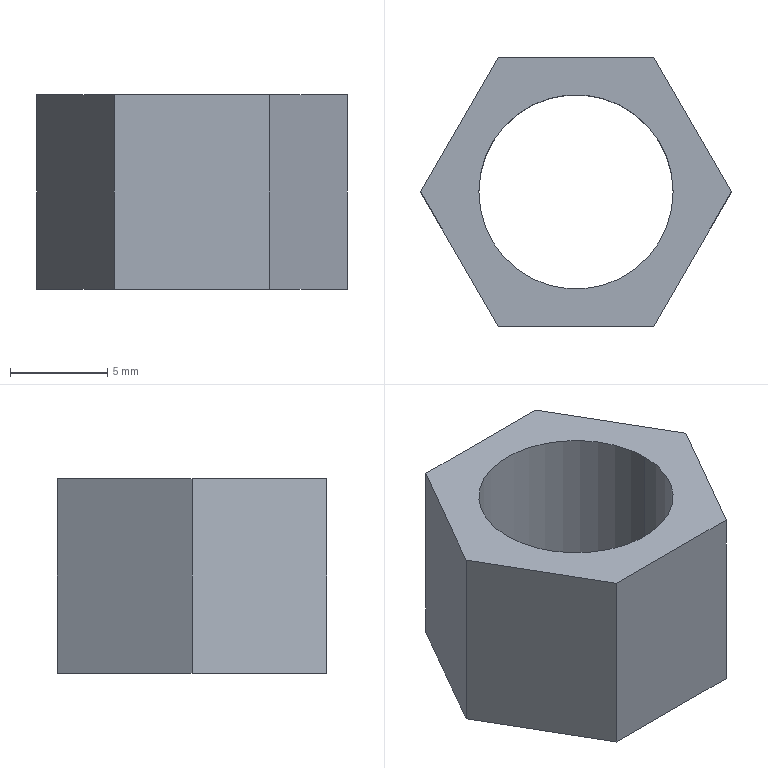Part | NX | features solid 2 | 1 solid | 10 faces | box 16 x 13.856 x 10 mm | volume 877.371 mm3 | plane 8 | cylinder 2 | commonest cylinder face diameters 10 x2
STEP:
#1=CARTESIAN_POINT('',(645.,-175.,1310.));
#2=VERTEX_POINT('',#1);
#3=CARTESIAN_POINT('',(655.,-175.,1310.));
#4=VERTEX_POINT('',#3);
#5=CARTESIAN_POINT('',(650.,-175.,1310.));
#6=DIRECTION('',(0.,0.,1.));
#7=DIRECTION('',(0.,1.,0.));
#8=AXIS2_PLACEMENT_3D('',#5,#6,#7);
#9=CIRCLE('',#8,5.);
#10=EDGE_CURVE('',#2,#4,#9,.T.);
#11=ORIENTED_EDGE('',*,*,#10,.F.);
#12=CARTESIAN_POINT('',(650.,-175.,1310.));
#13=DIRECTION('',(0.,0.,1.));
#14=DIRECTION('',(0.,1.,0.));
#15=AXIS2_PLACEMENT_3D('',#12,#13,#14);
#16=CIRCLE('',#15,5.);
#17=EDGE_CURVE('',#4,#2,#16,.T.);
#18=ORIENTED_EDGE('',*,*,#17,.F.);
#19=EDGE_LOOP('',(#11,#18));
#20=FACE_BOUND('',#19,.T.);
#21=CARTESIAN_POINT('',(646.,-168.072,1310.));
#22=VERTEX_POINT('',#21);
#23=CARTESIAN_POINT('',(654.,-168.072,1310.));
#24=VERTEX_POINT('',#23);
#25=CARTESIAN_POINT('',(646.,-168.072,1310.));
#26=DIRECTION('',(1.,0.,0.));
#27=VECTOR('',#26,1000.);
#28=LINE('',#25,#27);
#29=EDGE_CURVE('',#22,#24,#28,.T.);
#30=ORIENTED_EDGE('',*,*,#29,.F.);
#31=CARTESIAN_POINT('',(642.,-175.,1310.));
#32=VERTEX_POINT('',#31);
#33=CARTESIAN_POINT('',(642.,-175.,1310.));
#34=DIRECTION('',(0.5,0.866,0.));
#35=VECTOR('',#34,1000.);
#36=LINE('',#33,#35);
#37=EDGE_CURVE('',#32,#22,#36,.T.);
#38=ORIENTED_EDGE('',*,*,#37,.F.);
#39=CARTESIAN_POINT('',(646.,-181.928,1310.));
#40=VERTEX_POINT('',#39);
#41=CARTESIAN_POINT('',(646.,-181.928,1310.));
#42=DIRECTION('',(-0.5,0.866,0.));
#43=VECTOR('',#42,1000.);
#44=LINE('',#41,#43);
#45=EDGE_CURVE('',#40,#32,#44,.T.);
#46=ORIENTED_EDGE('',*,*,#45,.F.);
#47=CARTESIAN_POINT('',(654.,-181.928,1310.));
#48=VERTEX_POINT('',#47);
#49=CARTESIAN_POINT('',(654.,-181.928,1310.));
#50=DIRECTION('',(-1.,0.,0.));
#51=VECTOR('',#50,1000.);
#52=LINE('',#49,#51);
#53=EDGE_CURVE('',#48,#40,#52,.T.);
#54=ORIENTED_EDGE('',*,*,#53,.F.);
#55=CARTESIAN_POINT('',(658.,-175.,1310.));
#56=VERTEX_POINT('',#55);
#57=CARTESIAN_POINT('',(658.,-175.,1310.));
#58=DIRECTION('',(-0.5,-0.866,0.));
#59=VECTOR('',#58,1000.);
#60=LINE('',#57,#59);
#61=EDGE_CURVE('',#56,#48,#60,.T.);
#62=ORIENTED_EDGE('',*,*,#61,.F.);
#63=CARTESIAN_POINT('',(654.,-168.072,1310.));
#64=DIRECTION('',(0.5,-0.866,0.));
#65=VECTOR('',#64,1000.);
#66=LINE('',#63,#65);
#67=EDGE_CURVE('',#24,#56,#66,.T.);
#68=ORIENTED_EDGE('',*,*,#67,.F.);
#69=EDGE_LOOP('',(#30,#38,#46,#54,#62,#68));
#70=FACE_BOUND('',#69,.T.);
#71=CARTESIAN_POINT('',(650.,-325.,1310.));
#72=DIRECTION('',(0.,0.,-1.));
#73=DIRECTION('',(0.,-1.,0.));
#74=AXIS2_PLACEMENT_3D('',#71,#72,#73);
#75=PLANE('',#74);
#76=ADVANCED_FACE('',(#20,#70),#75,.F.);
#77=CARTESIAN_POINT('',(645.,-175.,1300.));
#78=VERTEX_POINT('',#77);
#79=CARTESIAN_POINT('',(655.,-175.,1300.));
#80=VERTEX_POINT('',#79);
#81=CARTESIAN_POINT('',(650.,-175.,1300.));
#82=DIRECTION('',(0.,0.,1.));
#83=DIRECTION('',(0.,1.,0.));
#84=AXIS2_PLACEMENT_3D('',#81,#82,#83);
#85=CIRCLE('',#84,5.);
#86=EDGE_CURVE('',#78,#80,#85,.T.);
#87=ORIENTED_EDGE('',*,*,#86,.T.);
#88=CARTESIAN_POINT('',(650.,-175.,1300.));
#89=DIRECTION('',(0.,0.,1.));
#90=DIRECTION('',(0.,1.,0.));
#91=AXIS2_PLACEMENT_3D('',#88,#89,#90);
#92=CIRCLE('',#91,5.);
#93=EDGE_CURVE('',#80,#78,#92,.T.);
#94=ORIENTED_EDGE('',*,*,#93,.T.);
#95=EDGE_LOOP('',(#87,#94));
#96=FACE_BOUND('',#95,.T.);
#97=CARTESIAN_POINT('',(646.,-168.072,1300.));
#98=VERTEX_POINT('',#97);
#99=CARTESIAN_POINT('',(654.,-168.072,1300.));
#100=VERTEX_POINT('',#99);
#101=CARTESIAN_POINT('',(646.,-168.072,1300.));
#102=DIRECTION('',(1.,0.,0.));
#103=VECTOR('',#102,1000.);
#104=LINE('',#101,#103);
#105=EDGE_CURVE('',#98,#100,#104,.T.);
#106=ORIENTED_EDGE('',*,*,#105,.T.);
#107=CARTESIAN_POINT('',(658.,-175.,1300.));
#108=VERTEX_POINT('',#107);
#109=CARTESIAN_POINT('',(654.,-168.072,1300.));
#110=DIRECTION('',(0.5,-0.866,0.));
#111=VECTOR('',#110,1000.);
#112=LINE('',#109,#111);
#113=EDGE_CURVE('',#100,#108,#112,.T.);
#114=ORIENTED_EDGE('',*,*,#113,.T.);
#115=CARTESIAN_POINT('',(654.,-181.928,1300.));
#116=VERTEX_POINT('',#115);
#117=CARTESIAN_POINT('',(658.,-175.,1300.));
#118=DIRECTION('',(-0.5,-0.866,0.));
#119=VECTOR('',#118,1000.);
#120=LINE('',#117,#119);
#121=EDGE_CURVE('',#108,#116,#120,.T.);
#122=ORIENTED_EDGE('',*,*,#121,.T.);
#123=CARTESIAN_POINT('',(646.,-181.928,1300.));
#124=VERTEX_POINT('',#123);
#125=CARTESIAN_POINT('',(654.,-181.928,1300.));
#126=DIRECTION('',(-1.,0.,0.));
#127=VECTOR('',#126,1000.);
#128=LINE('',#125,#127);
#129=EDGE_CURVE('',#116,#124,#128,.T.);
#130=ORIENTED_EDGE('',*,*,#129,.T.);
#131=CARTESIAN_POINT('',(642.,-175.,1300.));
#132=VERTEX_POINT('',#131);
#133=CARTESIAN_POINT('',(646.,-181.928,1300.));
#134=DIRECTION('',(-0.5,0.866,0.));
#135=VECTOR('',#134,1000.);
#136=LINE('',#133,#135);
#137=EDGE_CURVE('',#124,#132,#136,.T.);
#138=ORIENTED_EDGE('',*,*,#137,.T.);
#139=CARTESIAN_POINT('',(642.,-175.,1300.));
#140=DIRECTION('',(0.5,0.866,0.));
#141=VECTOR('',#140,1000.);
#142=LINE('',#139,#141);
#143=EDGE_CURVE('',#132,#98,#142,.T.);
#144=ORIENTED_EDGE('',*,*,#143,.T.);
#145=EDGE_LOOP('',(#106,#114,#122,#130,#138,#144));
#146=FACE_BOUND('',#145,.T.);
#147=CARTESIAN_POINT('',(650.,-325.,1300.));
#148=DIRECTION('',(0.,0.,-1.));
#149=DIRECTION('',(0.,-1.,0.));
#150=AXIS2_PLACEMENT_3D('',#147,#148,#149);
#151=PLANE('',#150);
#152=ADVANCED_FACE('',(#96,#146),#151,.T.);
#153=ORIENTED_EDGE('',*,*,#37,.T.);
#154=CARTESIAN_POINT('',(646.,-168.072,1300.));
#155=DIRECTION('',(0.,0.,1.));
#156=VECTOR('',#155,1000.);
#157=LINE('',#154,#156);
#158=EDGE_CURVE('',#98,#22,#157,.T.);
#159=ORIENTED_EDGE('',*,*,#158,.F.);
#160=ORIENTED_EDGE('',*,*,#143,.F.);
#161=CARTESIAN_POINT('',(642.,-175.,1300.));
#162=DIRECTION('',(0.,0.,1.));
#163=VECTOR('',#162,1000.);
#164=LINE('',#161,#163);
#165=EDGE_CURVE('',#132,#32,#164,.T.);
#166=ORIENTED_EDGE('',*,*,#165,.T.);
#167=EDGE_LOOP('',(#153,#159,#160,#166));
#168=FACE_BOUND('',#167,.T.);
#169=CARTESIAN_POINT('',(642.,-175.,1300.));
#170=DIRECTION('',(0.866,-0.5,0.));
#171=DIRECTION('',(0.,0.,-1.));
#172=AXIS2_PLACEMENT_3D('',#169,#170,#171);
#173=PLANE('',#172);
#174=ADVANCED_FACE('',(#168),#173,.F.);
#175=CARTESIAN_POINT('',(655.,-175.,1300.));
#176=DIRECTION('',(0.,0.,1.));
#177=VECTOR('',#176,1000.);
#178=LINE('',#175,#177);
#179=EDGE_CURVE('',#80,#4,#178,.T.);
#180=ORIENTED_EDGE('',*,*,#179,.F.);
#181=ORIENTED_EDGE('',*,*,#86,.F.);
#182=CARTESIAN_POINT('',(645.,-175.,1300.));
#183=DIRECTION('',(0.,0.,1.));
#184=VECTOR('',#183,1000.);
#185=LINE('',#182,#184);
#186=EDGE_CURVE('',#2,#78,#185,.F.);
#187=ORIENTED_EDGE('',*,*,#186,.F.);
#188=ORIENTED_EDGE('',*,*,#10,.T.);
#189=EDGE_LOOP('',(#180,#181,#187,#188));
#190=FACE_BOUND('',#189,.T.);
#191=CARTESIAN_POINT('',(650.,-175.,1300.));
#192=DIRECTION('',(0.,0.,1.));
#193=DIRECTION('',(-1.,0.,0.));
#194=AXIS2_PLACEMENT_3D('',#191,#192,#193);
#195=CYLINDRICAL_SURFACE('',#194,5.);
#196=ADVANCED_FACE('',(#190),#195,.F.);
#197=ORIENTED_EDGE('',*,*,#45,.T.);
#198=ORIENTED_EDGE('',*,*,#165,.F.);
#199=ORIENTED_EDGE('',*,*,#137,.F.);
#200=CARTESIAN_POINT('',(646.,-181.928,1300.));
#201=DIRECTION('',(0.,0.,1.));
#202=VECTOR('',#201,1000.);
#203=LINE('',#200,#202);
#204=EDGE_CURVE('',#124,#40,#203,.T.);
#205=ORIENTED_EDGE('',*,*,#204,.T.);
#206=EDGE_LOOP('',(#197,#198,#199,#205));
#207=FACE_BOUND('',#206,.T.);
#208=CARTESIAN_POINT('',(646.,-181.928,1300.));
#209=DIRECTION('',(0.866,0.5,0.));
#210=DIRECTION('',(0.,0.,-1.));
#211=AXIS2_PLACEMENT_3D('',#208,#209,#210);
#212=PLANE('',#211);
#213=ADVANCED_FACE('',(#207),#212,.F.);
#214=ORIENTED_EDGE('',*,*,#53,.T.);
#215=ORIENTED_EDGE('',*,*,#204,.F.);
#216=ORIENTED_EDGE('',*,*,#129,.F.);
#217=CARTESIAN_POINT('',(654.,-181.928,1300.));
#218=DIRECTION('',(0.,0.,1.));
#219=VECTOR('',#218,1000.);
#220=LINE('',#217,#219);
#221=EDGE_CURVE('',#116,#48,#220,.T.);
#222=ORIENTED_EDGE('',*,*,#221,.T.);
#223=EDGE_LOOP('',(#214,#215,#216,#222));
#224=FACE_BOUND('',#223,.T.);
#225=CARTESIAN_POINT('',(654.,-181.928,1300.));
#226=DIRECTION('',(0.,1.,0.));
#227=DIRECTION('',(1.,0.,0.));
#228=AXIS2_PLACEMENT_3D('',#225,#226,#227);
#229=PLANE('',#228);
#230=ADVANCED_FACE('',(#224),#229,.F.);
#231=ORIENTED_EDGE('',*,*,#61,.T.);
#232=ORIENTED_EDGE('',*,*,#221,.F.);
#233=ORIENTED_EDGE('',*,*,#121,.F.);
#234=CARTESIAN_POINT('',(658.,-175.,1300.));
#235=DIRECTION('',(0.,0.,1.));
#236=VECTOR('',#235,1000.);
#237=LINE('',#234,#236);
#238=EDGE_CURVE('',#108,#56,#237,.T.);
#239=ORIENTED_EDGE('',*,*,#238,.T.);
#240=EDGE_LOOP('',(#231,#232,#233,#239));
#241=FACE_BOUND('',#240,.T.);
#242=CARTESIAN_POINT('',(658.,-175.,1300.));
#243=DIRECTION('',(-0.866,0.5,0.));
#244=DIRECTION('',(0.,0.,1.));
#245=AXIS2_PLACEMENT_3D('',#242,#243,#244);
#246=PLANE('',#245);
#247=ADVANCED_FACE('',(#241),#246,.F.);
#248=ORIENTED_EDGE('',*,*,#67,.T.);
#249=ORIENTED_EDGE('',*,*,#238,.F.);
#250=ORIENTED_EDGE('',*,*,#113,.F.);
#251=CARTESIAN_POINT('',(654.,-168.072,1300.));
#252=DIRECTION('',(0.,0.,1.));
#253=VECTOR('',#252,1000.);
#254=LINE('',#251,#253);
#255=EDGE_CURVE('',#100,#24,#254,.T.);
#256=ORIENTED_EDGE('',*,*,#255,.T.);
#257=EDGE_LOOP('',(#248,#249,#250,#256));
#258=FACE_BOUND('',#257,.T.);
#259=CARTESIAN_POINT('',(654.,-168.072,1300.));
#260=DIRECTION('',(-0.866,-0.5,0.));
#261=DIRECTION('',(-0.5,0.866,0.));
#262=AXIS2_PLACEMENT_3D('',#259,#260,#261);
#263=PLANE('',#262);
#264=ADVANCED_FACE('',(#258),#263,.F.);
#265=ORIENTED_EDGE('',*,*,#29,.T.);
#266=ORIENTED_EDGE('',*,*,#255,.F.);
#267=ORIENTED_EDGE('',*,*,#105,.F.);
#268=ORIENTED_EDGE('',*,*,#158,.T.);
#269=EDGE_LOOP('',(#265,#266,#267,#268));
#270=FACE_BOUND('',#269,.T.);
#271=CARTESIAN_POINT('',(646.,-168.072,1300.));
#272=DIRECTION('',(0.,-1.,0.));
#273=DIRECTION('',(0.,0.,-1.));
#274=AXIS2_PLACEMENT_3D('',#271,#272,#273);
#275=PLANE('',#274);
#276=ADVANCED_FACE('',(#270),#275,.F.);
#277=ORIENTED_EDGE('',*,*,#93,.F.);
#278=ORIENTED_EDGE('',*,*,#179,.T.);
#279=ORIENTED_EDGE('',*,*,#17,.T.);
#280=ORIENTED_EDGE('',*,*,#186,.T.);
#281=EDGE_LOOP('',(#277,#278,#279,#280));
#282=FACE_BOUND('',#281,.T.);
#283=CARTESIAN_POINT('',(650.,-175.,1300.));
#284=DIRECTION('',(0.,0.,1.));
#285=DIRECTION('',(-1.,0.,0.));
#286=AXIS2_PLACEMENT_3D('',#283,#284,#285);
#287=CYLINDRICAL_SURFACE('',#286,5.);
#288=ADVANCED_FACE('',(#282),#287,.F.);
#289=CLOSED_SHELL('',(#76,#152,#174,#196,#213,#230,#247,#264,#276,#288));
#290=MANIFOLD_SOLID_BREP('',#289);
#291=(LENGTH_UNIT()NAMED_UNIT(*)SI_UNIT(.MILLI.,.METRE.));
#292=UNCERTAINTY_MEASURE_WITH_UNIT(LENGTH_MEASURE(0.00001),#291,'','');
#293=(NAMED_UNIT(*)PLANE_ANGLE_UNIT()SI_UNIT($,.RADIAN.));
#294=(NAMED_UNIT(*)SI_UNIT($,.STERADIAN.)SOLID_ANGLE_UNIT());
#295=(GEOMETRIC_REPRESENTATION_CONTEXT(3)GLOBAL_UNCERTAINTY_ASSIGNED_CONTEXT((#292))GLOBAL_UNIT_ASSIGNED_CONTEXT((#291,#293,#294))REPRESENTATION_CONTEXT('',''));
#296=ADVANCED_BREP_SHAPE_REPRESENTATION('',(#290),#295);